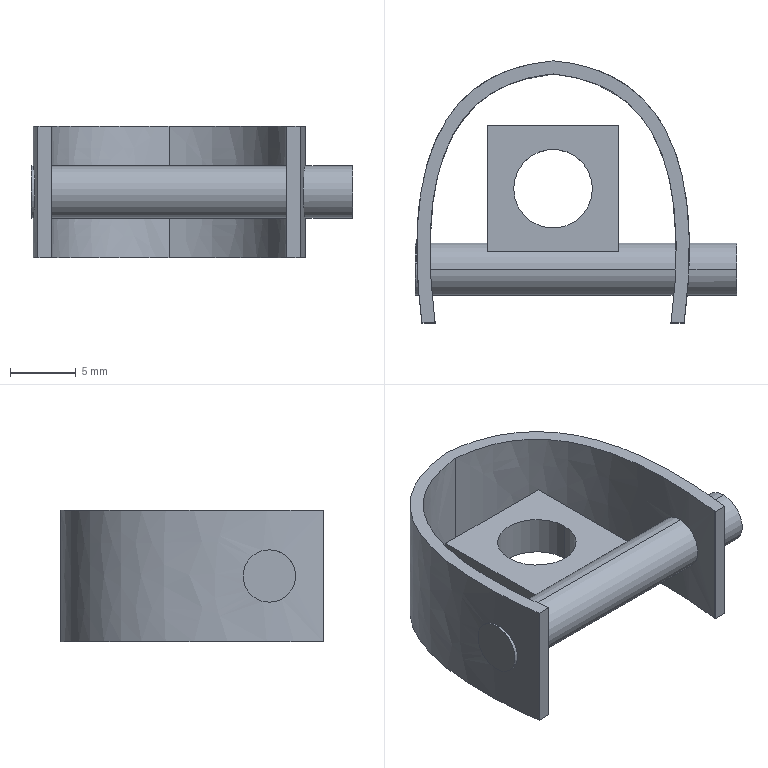Part | SolidWorks | features ICE 4, Extrusion 1 | 1 solid | 25 faces | box 24.5 x 20 x 10 mm | volume 968.354 mm3 | plane 11 | cylinder 10 | spline 4 | commonest cylinder face diameters 4 x6 6 x2 0.56 x1 0.938 x1
STEP:
#1=CARTESIAN_POINT('',(-3.,10.247,3.5));
#2=VERTEX_POINT('',#1);
#3=CARTESIAN_POINT('',(3.,10.247,3.5));
#4=VERTEX_POINT('',#3);
#5=CARTESIAN_POINT('',(0.,10.247,3.5));
#6=DIRECTION('',(0.,0.,1.));
#7=DIRECTION('',(1.,0.,0.));
#8=AXIS2_PLACEMENT_3D('',#5,#6,#7);
#9=CIRCLE('',#8,3.);
#10=EDGE_CURVE('',#2,#4,#9,.T.);
#11=ORIENTED_EDGE('',*,*,#10,.F.);
#12=CARTESIAN_POINT('',(-3.,10.247,6.5));
#13=VERTEX_POINT('',#12);
#14=CARTESIAN_POINT('',(-3.,10.247,-10.5));
#15=DIRECTION('',(0.,0.,1.));
#16=VECTOR('',#15,1000.);
#17=LINE('',#14,#16);
#18=EDGE_CURVE('',#2,#13,#17,.T.);
#19=ORIENTED_EDGE('',*,*,#18,.T.);
#20=CARTESIAN_POINT('',(3.,10.247,6.5));
#21=VERTEX_POINT('',#20);
#22=CARTESIAN_POINT('',(0.,10.247,6.5));
#23=DIRECTION('',(0.,0.,1.));
#24=DIRECTION('',(1.,0.,0.));
#25=AXIS2_PLACEMENT_3D('',#22,#23,#24);
#26=CIRCLE('',#25,3.);
#27=EDGE_CURVE('',#13,#21,#26,.T.);
#28=ORIENTED_EDGE('',*,*,#27,.T.);
#29=CARTESIAN_POINT('',(3.,10.247,-10.5));
#30=DIRECTION('',(0.,0.,1.));
#31=VECTOR('',#30,1000.);
#32=LINE('',#29,#31);
#33=EDGE_CURVE('',#4,#21,#32,.T.);
#34=ORIENTED_EDGE('',*,*,#33,.F.);
#35=EDGE_LOOP('',(#11,#19,#28,#34));
#36=FACE_OUTER_BOUND('',#35,.T.);
#37=CARTESIAN_POINT('',(0.,10.247,-10.5));
#38=DIRECTION('',(0.,0.,1.));
#39=DIRECTION('',(1.,0.,0.));
#40=AXIS2_PLACEMENT_3D('',#37,#38,#39);
#41=CYLINDRICAL_SURFACE('',#40,3.);
#42=ADVANCED_FACE('',(#36),#41,.F.);
#43=CARTESIAN_POINT('',(-10.5,4.102,7.));
#44=VERTEX_POINT('',#43);
#45=CARTESIAN_POINT('',(-10.5,4.102,3.));
#46=VERTEX_POINT('',#45);
#47=CARTESIAN_POINT('',(-10.5,4.102,5.));
#48=DIRECTION('',(-1.,0.,0.));
#49=DIRECTION('',(0.,0.,1.));
#50=AXIS2_PLACEMENT_3D('',#47,#48,#49);
#51=CIRCLE('',#50,2.);
#52=EDGE_CURVE('',#44,#46,#51,.T.);
#53=ORIENTED_EDGE('',*,*,#52,.F.);
#54=CARTESIAN_POINT('',(-10.36,4.102,7.));
#55=VERTEX_POINT('',#54);
#56=CARTESIAN_POINT('',(-10.5,4.102,7.));
#57=DIRECTION('',(1.,0.,0.));
#58=VECTOR('',#57,1000.);
#59=LINE('',#56,#58);
#60=EDGE_CURVE('',#44,#55,#59,.T.);
#61=ORIENTED_EDGE('',*,*,#60,.T.);
#62=CARTESIAN_POINT('',(-10.36,4.102,3.));
#63=VERTEX_POINT('',#62);
#64=CARTESIAN_POINT('',(-10.36,4.102,7.));
#65=CARTESIAN_POINT('',(-10.371,4.363,7.));
#66=CARTESIAN_POINT('',(-10.379,4.626,6.948));
#67=CARTESIAN_POINT('',(-10.39,5.107,6.749));
#68=CARTESIAN_POINT('',(-10.393,5.33,6.6));
#69=CARTESIAN_POINT('',(-10.395,5.607,6.323));
#70=CARTESIAN_POINT('',(-10.395,5.692,6.22));
#71=CARTESIAN_POINT('',(-10.394,5.837,6.003));
#72=CARTESIAN_POINT('',(-10.394,5.899,5.888));
#73=CARTESIAN_POINT('',(-10.393,5.999,5.646));
#74=CARTESIAN_POINT('',(-10.393,6.038,5.519));
#75=CARTESIAN_POINT('',(-10.392,6.089,5.263));
#76=CARTESIAN_POINT('',(-10.392,6.102,5.134));
#77=CARTESIAN_POINT('',(-10.392,6.102,4.87));
#78=CARTESIAN_POINT('',(-10.392,6.089,4.739));
#79=CARTESIAN_POINT('',(-10.393,6.039,4.484));
#80=CARTESIAN_POINT('',(-10.393,6.,4.357));
#81=CARTESIAN_POINT('',(-10.394,5.9,4.114));
#82=CARTESIAN_POINT('',(-10.394,5.839,3.999));
#83=CARTESIAN_POINT('',(-10.395,5.694,3.782));
#84=CARTESIAN_POINT('',(-10.395,5.609,3.679));
#85=CARTESIAN_POINT('',(-10.394,5.425,3.494));
#86=CARTESIAN_POINT('',(-10.393,5.324,3.411));
#87=CARTESIAN_POINT('',(-10.39,5.106,3.265));
#88=CARTESIAN_POINT('',(-10.388,4.989,3.203));
#89=CARTESIAN_POINT('',(-10.379,4.628,3.053));
#90=CARTESIAN_POINT('',(-10.371,4.366,3.));
#91=CARTESIAN_POINT('',(-10.36,4.102,3.));
#92=B_SPLINE_CURVE_WITH_KNOTS('',3,(#64,#65,#66,#67,#68,#69,#70,#71,#72,#73,#74,#75,#76,#77,#78,#79,#80,#81,#82,#83,#84,#85,#86,#87,#88,#89,#90,#91),.UNSPECIFIED.,.F.,.F.,(4,2,2,2,2,2,2,2,2,2,2,2,2,4),(0.006259,0.007041,0.007822,0.008213,0.008604,0.008994,0.009385,0.009776,0.01017,0.01056,0.01095,0.01134,0.01173,0.01251),.UNSPECIFIED.);
#93=EDGE_CURVE('',#55,#63,#92,.T.);
#94=ORIENTED_EDGE('',*,*,#93,.T.);
#95=CARTESIAN_POINT('',(-10.5,4.102,3.));
#96=DIRECTION('',(1.,0.,0.));
#97=VECTOR('',#96,1000.);
#98=LINE('',#95,#97);
#99=EDGE_CURVE('',#46,#63,#98,.T.);
#100=ORIENTED_EDGE('',*,*,#99,.F.);
#101=EDGE_LOOP('',(#53,#61,#94,#100));
#102=FACE_OUTER_BOUND('',#101,.T.);
#103=CARTESIAN_POINT('',(-10.5,4.102,5.));
#104=DIRECTION('',(1.,0.,0.));
#105=DIRECTION('',(0.,0.,-1.));
#106=AXIS2_PLACEMENT_3D('',#103,#104,#105);
#107=CYLINDRICAL_SURFACE('',#106,2.);
#108=ADVANCED_FACE('',(#102),#107,.T.);
#109=CARTESIAN_POINT('',(5.,5.425,6.5));
#110=VERTEX_POINT('',#109);
#111=CARTESIAN_POINT('',(5.,5.425,3.5));
#112=VERTEX_POINT('',#111);
#113=CARTESIAN_POINT('',(5.,4.102,5.));
#114=DIRECTION('',(-1.,0.,0.));
#115=DIRECTION('',(0.,-1.,0.));
#116=AXIS2_PLACEMENT_3D('',#113,#114,#115);
#117=CIRCLE('',#116,2.);
#118=EDGE_CURVE('',#110,#112,#117,.T.);
#119=ORIENTED_EDGE('',*,*,#118,.F.);
#120=CARTESIAN_POINT('',(-5.,5.425,6.5));
#121=VERTEX_POINT('',#120);
#122=CARTESIAN_POINT('',(14.,5.425,6.5));
#123=DIRECTION('',(-1.,0.,0.));
#124=VECTOR('',#123,1000.);
#125=LINE('',#122,#124);
#126=EDGE_CURVE('',#110,#121,#125,.T.);
#127=ORIENTED_EDGE('',*,*,#126,.T.);
#128=CARTESIAN_POINT('',(-5.,5.425,3.5));
#129=VERTEX_POINT('',#128);
#130=CARTESIAN_POINT('',(-5.,4.102,5.));
#131=DIRECTION('',(1.,0.,0.));
#132=DIRECTION('',(0.,1.,0.));
#133=AXIS2_PLACEMENT_3D('',#130,#131,#132);
#134=CIRCLE('',#133,2.);
#135=EDGE_CURVE('',#129,#121,#134,.T.);
#136=ORIENTED_EDGE('',*,*,#135,.F.);
#137=CARTESIAN_POINT('',(14.,5.425,3.5));
#138=DIRECTION('',(-1.,0.,0.));
#139=VECTOR('',#138,1000.);
#140=LINE('',#137,#139);
#141=EDGE_CURVE('',#112,#129,#140,.T.);
#142=ORIENTED_EDGE('',*,*,#141,.F.);
#143=EDGE_LOOP('',(#119,#127,#136,#142));
#144=FACE_BOUND('',#143,.T.);
#145=CARTESIAN_POINT('',(9.359,4.102,7.));
#146=VERTEX_POINT('',#145);
#147=CARTESIAN_POINT('',(9.359,4.102,3.));
#148=VERTEX_POINT('',#147);
#149=CARTESIAN_POINT('',(9.359,4.102,7.));
#150=CARTESIAN_POINT('',(9.365,4.234,7.));
#151=CARTESIAN_POINT('',(9.37,4.364,6.987));
#152=CARTESIAN_POINT('',(9.378,4.619,6.936));
#153=CARTESIAN_POINT('',(9.382,4.746,6.898));
#154=CARTESIAN_POINT('',(9.388,4.989,6.797));
#155=CARTESIAN_POINT('',(9.39,5.103,6.736));
#156=CARTESIAN_POINT('',(9.393,5.321,6.591));
#157=CARTESIAN_POINT('',(9.394,5.424,6.506));
#158=CARTESIAN_POINT('',(9.395,5.701,6.23));
#159=CARTESIAN_POINT('',(9.394,5.85,6.006));
#160=CARTESIAN_POINT('',(9.393,6.049,5.525));
#161=CARTESIAN_POINT('',(9.392,6.102,5.262));
#162=CARTESIAN_POINT('',(9.392,6.102,4.87));
#163=CARTESIAN_POINT('',(9.392,6.089,4.738));
#164=CARTESIAN_POINT('',(9.393,6.038,4.481));
#165=CARTESIAN_POINT('',(9.393,6.,4.356));
#166=CARTESIAN_POINT('',(9.394,5.9,4.114));
#167=CARTESIAN_POINT('',(9.394,5.837,3.997));
#168=CARTESIAN_POINT('',(9.395,5.692,3.78));
#169=CARTESIAN_POINT('',(9.395,5.61,3.679));
#170=CARTESIAN_POINT('',(9.394,5.423,3.493));
#171=CARTESIAN_POINT('',(9.393,5.322,3.41));
#172=CARTESIAN_POINT('',(9.39,5.105,3.265));
#173=CARTESIAN_POINT('',(9.388,4.988,3.202));
#174=CARTESIAN_POINT('',(9.382,4.746,3.102));
#175=CARTESIAN_POINT('',(9.378,4.621,3.064));
#176=CARTESIAN_POINT('',(9.37,4.365,3.013));
#177=CARTESIAN_POINT('',(9.365,4.232,3.));
#178=CARTESIAN_POINT('',(9.359,4.102,3.));
#179=B_SPLINE_CURVE_WITH_KNOTS('',3,(#149,#150,#151,#152,#153,#154,#155,#156,#157,#158,#159,#160,#161,#162,#163,#164,#165,#166,#167,#168,#169,#170,#171,#172,#173,#174,#175,#176,#177,#178),.UNSPECIFIED.,.F.,.F.,(4,2,2,2,2,2,2,2,2,2,2,2,2,2,4),(0.,0.0003909,0.0007817,0.001173,0.001563,0.002345,0.003127,0.003518,0.003909,0.0043,0.00469,0.005081,0.005472,0.005863,0.006254),.UNSPECIFIED.);
#180=EDGE_CURVE('',#146,#148,#179,.T.);
#181=ORIENTED_EDGE('',*,*,#180,.T.);
#182=CARTESIAN_POINT('',(-9.359,4.102,3.));
#183=VERTEX_POINT('',#182);
#184=CARTESIAN_POINT('',(14.,4.102,3.));
#185=DIRECTION('',(-1.,0.,0.));
#186=VECTOR('',#185,1000.);
#187=LINE('',#184,#186);
#188=EDGE_CURVE('',#148,#183,#187,.T.);
#189=ORIENTED_EDGE('',*,*,#188,.T.);
#190=CARTESIAN_POINT('',(-9.359,4.102,7.));
#191=VERTEX_POINT('',#190);
#192=CARTESIAN_POINT('',(-9.359,4.102,3.));
#193=CARTESIAN_POINT('',(-9.365,4.234,3.));
#194=CARTESIAN_POINT('',(-9.37,4.364,3.013));
#195=CARTESIAN_POINT('',(-9.378,4.619,3.064));
#196=CARTESIAN_POINT('',(-9.382,4.746,3.102));
#197=CARTESIAN_POINT('',(-9.388,4.989,3.203));
#198=CARTESIAN_POINT('',(-9.39,5.103,3.264));
#199=CARTESIAN_POINT('',(-9.393,5.321,3.409));
#200=CARTESIAN_POINT('',(-9.394,5.424,3.494));
#201=CARTESIAN_POINT('',(-9.395,5.701,3.77));
#202=CARTESIAN_POINT('',(-9.394,5.85,3.994));
#203=CARTESIAN_POINT('',(-9.393,6.049,4.475));
#204=CARTESIAN_POINT('',(-9.392,6.102,4.738));
#205=CARTESIAN_POINT('',(-9.392,6.102,5.13));
#206=CARTESIAN_POINT('',(-9.392,6.089,5.262));
#207=CARTESIAN_POINT('',(-9.393,6.038,5.519));
#208=CARTESIAN_POINT('',(-9.393,6.,5.644));
#209=CARTESIAN_POINT('',(-9.394,5.9,5.886));
#210=CARTESIAN_POINT('',(-9.394,5.837,6.003));
#211=CARTESIAN_POINT('',(-9.395,5.692,6.22));
#212=CARTESIAN_POINT('',(-9.395,5.61,6.321));
#213=CARTESIAN_POINT('',(-9.394,5.423,6.507));
#214=CARTESIAN_POINT('',(-9.393,5.322,6.59));
#215=CARTESIAN_POINT('',(-9.39,5.105,6.735));
#216=CARTESIAN_POINT('',(-9.388,4.988,6.798));
#217=CARTESIAN_POINT('',(-9.382,4.746,6.898));
#218=CARTESIAN_POINT('',(-9.378,4.621,6.936));
#219=CARTESIAN_POINT('',(-9.37,4.365,6.987));
#220=CARTESIAN_POINT('',(-9.365,4.232,7.));
#221=CARTESIAN_POINT('',(-9.359,4.102,7.));
#222=B_SPLINE_CURVE_WITH_KNOTS('',3,(#192,#193,#194,#195,#196,#197,#198,#199,#200,#201,#202,#203,#204,#205,#206,#207,#208,#209,#210,#211,#212,#213,#214,#215,#216,#217,#218,#219,#220,#221),.UNSPECIFIED.,.F.,.F.,(4,2,2,2,2,2,2,2,2,2,2,2,2,2,4),(0.,0.0003909,0.0007817,0.001173,0.001563,0.002345,0.003127,0.003518,0.003909,0.0043,0.00469,0.005081,0.005472,0.005863,0.006254),.UNSPECIFIED.);
#223=EDGE_CURVE('',#183,#191,#222,.T.);
#224=ORIENTED_EDGE('',*,*,#223,.T.);
#225=CARTESIAN_POINT('',(14.,4.102,7.));
#226=DIRECTION('',(-1.,0.,0.));
#227=VECTOR('',#226,1000.);
#228=LINE('',#225,#227);
#229=EDGE_CURVE('',#146,#191,#228,.T.);
#230=ORIENTED_EDGE('',*,*,#229,.F.);
#231=EDGE_LOOP('',(#181,#189,#224,#230));
#232=FACE_OUTER_BOUND('',#231,.T.);
#233=CARTESIAN_POINT('',(14.,4.102,5.));
#234=DIRECTION('',(-1.,0.,0.));
#235=DIRECTION('',(0.,0.,1.));
#236=AXIS2_PLACEMENT_3D('',#233,#234,#235);
#237=CYLINDRICAL_SURFACE('',#236,2.);
#238=ADVANCED_FACE('',(#144,#232),#237,.T.);
#239=CARTESIAN_POINT('',(14.,4.102,3.));
#240=VERTEX_POINT('',#239);
#241=CARTESIAN_POINT('',(14.,4.102,7.));
#242=VERTEX_POINT('',#241);
#243=CARTESIAN_POINT('',(14.,4.102,5.));
#244=DIRECTION('',(1.,0.,0.));
#245=DIRECTION('',(0.,0.,-1.));
#246=AXIS2_PLACEMENT_3D('',#243,#244,#245);
#247=CIRCLE('',#246,2.);
#248=EDGE_CURVE('',#240,#242,#247,.T.);
#249=ORIENTED_EDGE('',*,*,#248,.F.);
#250=CARTESIAN_POINT('',(10.36,4.102,3.));
#251=VERTEX_POINT('',#250);
#252=CARTESIAN_POINT('',(14.,4.102,3.));
#253=DIRECTION('',(-1.,0.,0.));
#254=VECTOR('',#253,1000.);
#255=LINE('',#252,#254);
#256=EDGE_CURVE('',#240,#251,#255,.T.);
#257=ORIENTED_EDGE('',*,*,#256,.T.);
#258=CARTESIAN_POINT('',(10.36,4.102,7.));
#259=VERTEX_POINT('',#258);
#260=CARTESIAN_POINT('',(10.36,4.102,3.));
#261=CARTESIAN_POINT('',(10.371,4.363,3.));
#262=CARTESIAN_POINT('',(10.379,4.626,3.052));
#263=CARTESIAN_POINT('',(10.39,5.107,3.251));
#264=CARTESIAN_POINT('',(10.393,5.33,3.4));
#265=CARTESIAN_POINT('',(10.395,5.607,3.677));
#266=CARTESIAN_POINT('',(10.395,5.692,3.78));
#267=CARTESIAN_POINT('',(10.394,5.837,3.997));
#268=CARTESIAN_POINT('',(10.394,5.899,4.112));
#269=CARTESIAN_POINT('',(10.393,5.999,4.354));
#270=CARTESIAN_POINT('',(10.393,6.038,4.481));
#271=CARTESIAN_POINT('',(10.392,6.089,4.737));
#272=CARTESIAN_POINT('',(10.392,6.102,4.866));
#273=CARTESIAN_POINT('',(10.392,6.102,5.13));
#274=CARTESIAN_POINT('',(10.392,6.089,5.261));
#275=CARTESIAN_POINT('',(10.393,6.039,5.516));
#276=CARTESIAN_POINT('',(10.393,6.,5.643));
#277=CARTESIAN_POINT('',(10.394,5.9,5.886));
#278=CARTESIAN_POINT('',(10.394,5.839,6.001));
#279=CARTESIAN_POINT('',(10.395,5.694,6.218));
#280=CARTESIAN_POINT('',(10.395,5.609,6.321));
#281=CARTESIAN_POINT('',(10.394,5.425,6.506));
#282=CARTESIAN_POINT('',(10.393,5.324,6.589));
#283=CARTESIAN_POINT('',(10.39,5.106,6.735));
#284=CARTESIAN_POINT('',(10.388,4.989,6.797));
#285=CARTESIAN_POINT('',(10.379,4.628,6.947));
#286=CARTESIAN_POINT('',(10.371,4.366,7.));
#287=CARTESIAN_POINT('',(10.36,4.102,7.));
#288=B_SPLINE_CURVE_WITH_KNOTS('',3,(#260,#261,#262,#263,#264,#265,#266,#267,#268,#269,#270,#271,#272,#273,#274,#275,#276,#277,#278,#279,#280,#281,#282,#283,#284,#285,#286,#287),.UNSPECIFIED.,.F.,.F.,(4,2,2,2,2,2,2,2,2,2,2,2,2,4),(0.006259,0.007041,0.007822,0.008213,0.008604,0.008994,0.009385,0.009776,0.01017,0.01056,0.01095,0.01134,0.01173,0.01251),.UNSPECIFIED.);
#289=EDGE_CURVE('',#251,#259,#288,.T.);
#290=ORIENTED_EDGE('',*,*,#289,.T.);
#291=CARTESIAN_POINT('',(14.,4.102,7.));
#292=DIRECTION('',(-1.,0.,0.));
#293=VECTOR('',#292,1000.);
#294=LINE('',#291,#293);
#295=EDGE_CURVE('',#242,#259,#294,.T.);
#296=ORIENTED_EDGE('',*,*,#295,.F.);
#297=EDGE_LOOP('',(#249,#257,#290,#296));
#298=FACE_OUTER_BOUND('',#297,.T.);
#299=CARTESIAN_POINT('',(14.,4.102,5.));
#300=DIRECTION('',(-1.,0.,0.));
#301=DIRECTION('',(0.,0.,1.));
#302=AXIS2_PLACEMENT_3D('',#299,#300,#301);
#303=CYLINDRICAL_SURFACE('',#302,2.);
#304=ADVANCED_FACE('',(#298),#303,.T.);
#305=CARTESIAN_POINT('',(0.,20.,0.));
#306=VERTEX_POINT('',#305);
#307=CARTESIAN_POINT('',(-10.,0.,0.));
#308=VERTEX_POINT('',#307);
#309=CARTESIAN_POINT('',(0.,20.,0.));
#310=CARTESIAN_POINT('',(-12.419,18.909,0.));
#311=CARTESIAN_POINT('',(-10.,0.,0.));
#312=B_SPLINE_CURVE_WITH_KNOTS('',2,(#309,#310,#311),.UNSPECIFIED.,.F.,.F.,(3,3),(0.,1.),.UNSPECIFIED.);
#313=EDGE_CURVE('',#306,#308,#312,.T.);
#314=ORIENTED_EDGE('',*,*,#313,.T.);
#315=CARTESIAN_POINT('',(-10.,0.,10.));
#316=VERTEX_POINT('',#315);
#317=CARTESIAN_POINT('',(-10.,0.,10.));
#318=DIRECTION('',(0.,0.,-1.));
#319=VECTOR('',#318,1000.);
#320=LINE('',#317,#319);
#321=EDGE_CURVE('',#316,#308,#320,.T.);
#322=ORIENTED_EDGE('',*,*,#321,.F.);
#323=CARTESIAN_POINT('',(0.,20.,10.));
#324=VERTEX_POINT('',#323);
#325=CARTESIAN_POINT('',(0.,20.,10.));
#326=CARTESIAN_POINT('',(-12.419,18.909,10.));
#327=CARTESIAN_POINT('',(-10.,0.,10.));
#328=B_SPLINE_CURVE_WITH_KNOTS('',2,(#325,#326,#327),.UNSPECIFIED.,.F.,.F.,(3,3),(0.,1.),.UNSPECIFIED.);
#329=EDGE_CURVE('',#324,#316,#328,.T.);
#330=ORIENTED_EDGE('',*,*,#329,.F.);
#331=CARTESIAN_POINT('',(0.,20.,10.));
#332=DIRECTION('',(0.,0.,-1.));
#333=VECTOR('',#332,1000.);
#334=LINE('',#331,#333);
#335=EDGE_CURVE('',#324,#306,#334,.T.);
#336=ORIENTED_EDGE('',*,*,#335,.T.);
#337=EDGE_LOOP('',(#314,#322,#330,#336));
#338=FACE_OUTER_BOUND('',#337,.T.);
#339=CARTESIAN_POINT('',(-10.36,4.102,3.));
#340=CARTESIAN_POINT('',(-10.354,3.97,3.));
#341=CARTESIAN_POINT('',(-10.348,3.84,3.013));
#342=CARTESIAN_POINT('',(-10.335,3.584,3.064));
#343=CARTESIAN_POINT('',(-10.327,3.457,3.102));
#344=CARTESIAN_POINT('',(-10.313,3.215,3.203));
#345=CARTESIAN_POINT('',(-10.305,3.1,3.264));
#346=CARTESIAN_POINT('',(-10.29,2.883,3.409));
#347=CARTESIAN_POINT('',(-10.283,2.78,3.493));
#348=CARTESIAN_POINT('',(-10.262,2.503,3.77));
#349=CARTESIAN_POINT('',(-10.25,2.354,3.993));
#350=CARTESIAN_POINT('',(-10.233,2.155,4.475));
#351=CARTESIAN_POINT('',(-10.228,2.102,4.738));
#352=CARTESIAN_POINT('',(-10.228,2.102,5.13));
#353=CARTESIAN_POINT('',(-10.229,2.115,5.262));
#354=CARTESIAN_POINT('',(-10.234,2.166,5.519));
#355=CARTESIAN_POINT('',(-10.237,2.204,5.644));
#356=CARTESIAN_POINT('',(-10.245,2.304,5.886));
#357=CARTESIAN_POINT('',(-10.251,2.367,6.003));
#358=CARTESIAN_POINT('',(-10.262,2.512,6.22));
#359=CARTESIAN_POINT('',(-10.269,2.594,6.321));
#360=CARTESIAN_POINT('',(-10.283,2.781,6.508));
#361=CARTESIAN_POINT('',(-10.29,2.882,6.59));
#362=CARTESIAN_POINT('',(-10.305,3.099,6.735));
#363=CARTESIAN_POINT('',(-10.313,3.216,6.798));
#364=CARTESIAN_POINT('',(-10.327,3.458,6.898));
#365=CARTESIAN_POINT('',(-10.335,3.583,6.936));
#366=CARTESIAN_POINT('',(-10.348,3.839,6.987));
#367=CARTESIAN_POINT('',(-10.354,3.971,7.));
#368=CARTESIAN_POINT('',(-10.36,4.102,7.));
#369=B_SPLINE_CURVE_WITH_KNOTS('',3,(#339,#340,#341,#342,#343,#344,#345,#346,#347,#348,#349,#350,#351,#352,#353,#354,#355,#356,#357,#358,#359,#360,#361,#362,#363,#364,#365,#366,#367,#368),.UNSPECIFIED.,.F.,.F.,(4,2,2,2,2,2,2,2,2,2,2,2,2,2,4),(0.,0.0003912,0.0007824,0.001174,0.001565,0.002347,0.00313,0.003521,0.003912,0.004303,0.004694,0.005086,0.005477,0.005868,0.006259),.UNSPECIFIED.);
#370=EDGE_CURVE('',#63,#55,#369,.T.);
#371=ORIENTED_EDGE('',*,*,#370,.F.);
#372=ORIENTED_EDGE('',*,*,#93,.F.);
#373=EDGE_LOOP('',(#371,#372));
#374=FACE_BOUND('',#373,.T.);
#375=CARTESIAN_POINT('',(0.,20.,10.));
#376=CARTESIAN_POINT('',(0.,20.,0.));
#377=CARTESIAN_POINT('',(-12.419,18.909,10.));
#378=CARTESIAN_POINT('',(-12.419,18.909,0.));
#379=CARTESIAN_POINT('',(-10.,0.,10.));
#380=CARTESIAN_POINT('',(-10.,0.,0.));
#381=B_SPLINE_SURFACE_WITH_KNOTS('',2,1,((#375,#376),(#377,#378),(#379,#380)),.UNSPECIFIED.,.F.,.F.,.F.,(3,3),(2,2),(0.,1.),(0.,1.),.UNSPECIFIED.);
#382=ADVANCED_FACE('',(#338,#374),#381,.F.);
#383=CARTESIAN_POINT('',(-9.008,0.1269,0.));
#384=VERTEX_POINT('',#383);
#385=CARTESIAN_POINT('',(0.,18.996,0.));
#386=VERTEX_POINT('',#385);
#387=CARTESIAN_POINT('',(-9.008,0.1269,0.));
#388=CARTESIAN_POINT('',(-9.057,0.5062,0.));
#389=CARTESIAN_POINT('',(-9.147,1.275,0.));
#390=CARTESIAN_POINT('',(-9.287,2.741,0.));
#391=CARTESIAN_POINT('',(-9.392,4.492,0.));
#392=CARTESIAN_POINT('',(-9.405,6.444,0.));
#393=CARTESIAN_POINT('',(-9.274,8.852,0.));
#394=CARTESIAN_POINT('',(-8.837,11.493,0.));
#395=CARTESIAN_POINT('',(-7.897,14.069,0.));
#396=CARTESIAN_POINT('',(-6.57,16.069,0.));
#397=CARTESIAN_POINT('',(-4.863,17.548,0.));
#398=CARTESIAN_POINT('',(-3.071,18.387,0.));
#399=CARTESIAN_POINT('',(-1.41,18.817,0.));
#400=CARTESIAN_POINT('',(-0.463,18.953,0.));
#401=CARTESIAN_POINT('',(0.,18.996,0.));
#402=B_SPLINE_CURVE_WITH_KNOTS('',3,(#387,#388,#389,#390,#391,#392,#393,#394,#395,#396,#397,#398,#399,#400,#401),.UNSPECIFIED.,.F.,.F.,(4,1,1,1,1,1,1,1,1,1,1,1,4),(0.003764,0.0349,0.06603,0.1283,0.1906,0.2528,0.3774,0.5019,0.6264,0.7509,0.8755,0.9377,1.),.UNSPECIFIED.);
#403=EDGE_CURVE('',#384,#386,#402,.T.);
#404=ORIENTED_EDGE('',*,*,#403,.T.);
#405=CARTESIAN_POINT('',(0.,18.996,10.));
#406=VERTEX_POINT('',#405);
#407=CARTESIAN_POINT('',(0.,18.996,10.));
#408=DIRECTION('',(0.,0.,-1.));
#409=VECTOR('',#408,1000.);
#410=LINE('',#407,#409);
#411=EDGE_CURVE('',#406,#386,#410,.T.);
#412=ORIENTED_EDGE('',*,*,#411,.F.);
#413=CARTESIAN_POINT('',(-9.008,0.1269,10.));
#414=VERTEX_POINT('',#413);
#415=CARTESIAN_POINT('',(-9.008,0.1269,10.));
#416=CARTESIAN_POINT('',(-9.057,0.5062,10.));
#417=CARTESIAN_POINT('',(-9.147,1.275,10.));
#418=CARTESIAN_POINT('',(-9.287,2.741,10.));
#419=CARTESIAN_POINT('',(-9.392,4.492,10.));
#420=CARTESIAN_POINT('',(-9.405,6.444,10.));
#421=CARTESIAN_POINT('',(-9.274,8.852,10.));
#422=CARTESIAN_POINT('',(-8.837,11.493,10.));
#423=CARTESIAN_POINT('',(-7.897,14.069,10.));
#424=CARTESIAN_POINT('',(-6.57,16.069,10.));
#425=CARTESIAN_POINT('',(-4.863,17.548,10.));
#426=CARTESIAN_POINT('',(-3.071,18.387,10.));
#427=CARTESIAN_POINT('',(-1.41,18.817,10.));
#428=CARTESIAN_POINT('',(-0.463,18.953,10.));
#429=CARTESIAN_POINT('',(0.,18.996,10.));
#430=B_SPLINE_CURVE_WITH_KNOTS('',3,(#415,#416,#417,#418,#419,#420,#421,#422,#423,#424,#425,#426,#427,#428,#429),.UNSPECIFIED.,.F.,.F.,(4,1,1,1,1,1,1,1,1,1,1,1,4),(0.003764,0.0349,0.06603,0.1283,0.1906,0.2528,0.3774,0.5019,0.6264,0.7509,0.8755,0.9377,1.),.UNSPECIFIED.);
#431=EDGE_CURVE('',#414,#406,#430,.T.);
#432=ORIENTED_EDGE('',*,*,#431,.F.);
#433=CARTESIAN_POINT('',(-9.008,0.1269,10.));
#434=DIRECTION('',(0.,0.,-1.));
#435=VECTOR('',#434,1000.);
#436=LINE('',#433,#435);
#437=EDGE_CURVE('',#414,#384,#436,.T.);
#438=ORIENTED_EDGE('',*,*,#437,.T.);
#439=EDGE_LOOP('',(#404,#412,#432,#438));
#440=FACE_OUTER_BOUND('',#439,.T.);
#441=CARTESIAN_POINT('',(-9.359,4.102,7.));
#442=CARTESIAN_POINT('',(-9.347,3.841,7.));
#443=CARTESIAN_POINT('',(-9.333,3.578,6.948));
#444=CARTESIAN_POINT('',(-9.303,3.097,6.749));
#445=CARTESIAN_POINT('',(-9.287,2.874,6.6));
#446=CARTESIAN_POINT('',(-9.266,2.597,6.324));
#447=CARTESIAN_POINT('',(-9.259,2.512,6.221));
#448=CARTESIAN_POINT('',(-9.247,2.367,6.004));
#449=CARTESIAN_POINT('',(-9.242,2.305,5.889));
#450=CARTESIAN_POINT('',(-9.233,2.205,5.647));
#451=CARTESIAN_POINT('',(-9.23,2.166,5.52));
#452=CARTESIAN_POINT('',(-9.225,2.115,5.264));
#453=CARTESIAN_POINT('',(-9.224,2.102,5.134));
#454=CARTESIAN_POINT('',(-9.224,2.102,4.87));
#455=CARTESIAN_POINT('',(-9.225,2.115,4.739));
#456=CARTESIAN_POINT('',(-9.23,2.165,4.483));
#457=CARTESIAN_POINT('',(-9.233,2.204,4.356));
#458=CARTESIAN_POINT('',(-9.242,2.304,4.114));
#459=CARTESIAN_POINT('',(-9.247,2.366,3.999));
#460=CARTESIAN_POINT('',(-9.259,2.511,3.782));
#461=CARTESIAN_POINT('',(-9.266,2.595,3.679));
#462=CARTESIAN_POINT('',(-9.28,2.779,3.494));
#463=CARTESIAN_POINT('',(-9.287,2.88,3.411));
#464=CARTESIAN_POINT('',(-9.303,3.098,3.265));
#465=CARTESIAN_POINT('',(-9.311,3.215,3.203));
#466=CARTESIAN_POINT('',(-9.333,3.575,3.053));
#467=CARTESIAN_POINT('',(-9.347,3.838,3.));
#468=CARTESIAN_POINT('',(-9.359,4.102,3.));
#469=B_SPLINE_CURVE_WITH_KNOTS('',3,(#441,#442,#443,#444,#445,#446,#447,#448,#449,#450,#451,#452,#453,#454,#455,#456,#457,#458,#459,#460,#461,#462,#463,#464,#465,#466,#467,#468),.UNSPECIFIED.,.F.,.F.,(4,2,2,2,2,2,2,2,2,2,2,2,2,4),(0.006254,0.007036,0.007819,0.00821,0.008601,0.008992,0.009383,0.009774,0.01017,0.01056,0.01095,0.01134,0.01173,0.01251),.UNSPECIFIED.);
#470=EDGE_CURVE('',#191,#183,#469,.T.);
#471=ORIENTED_EDGE('',*,*,#470,.F.);
#472=ORIENTED_EDGE('',*,*,#223,.F.);
#473=EDGE_LOOP('',(#471,#472));
#474=FACE_BOUND('',#473,.T.);
#475=CARTESIAN_POINT('',(-9.008,0.1269,10.));
#476=CARTESIAN_POINT('',(-9.008,0.1269,0.));
#477=CARTESIAN_POINT('',(-9.057,0.5062,10.));
#478=CARTESIAN_POINT('',(-9.057,0.5062,0.));
#479=CARTESIAN_POINT('',(-9.147,1.275,10.));
#480=CARTESIAN_POINT('',(-9.147,1.275,0.));
#481=CARTESIAN_POINT('',(-9.287,2.741,10.));
#482=CARTESIAN_POINT('',(-9.287,2.741,0.));
#483=CARTESIAN_POINT('',(-9.392,4.492,10.));
#484=CARTESIAN_POINT('',(-9.392,4.492,0.));
#485=CARTESIAN_POINT('',(-9.405,6.444,10.));
#486=CARTESIAN_POINT('',(-9.405,6.444,0.));
#487=CARTESIAN_POINT('',(-9.274,8.852,10.));
#488=CARTESIAN_POINT('',(-9.274,8.852,0.));
#489=CARTESIAN_POINT('',(-8.837,11.493,10.));
#490=CARTESIAN_POINT('',(-8.837,11.493,0.));
#491=CARTESIAN_POINT('',(-7.897,14.069,10.));
#492=CARTESIAN_POINT('',(-7.897,14.069,0.));
#493=CARTESIAN_POINT('',(-6.57,16.069,10.));
#494=CARTESIAN_POINT('',(-6.57,16.069,0.));
#495=CARTESIAN_POINT('',(-4.863,17.548,10.));
#496=CARTESIAN_POINT('',(-4.863,17.548,0.));
#497=CARTESIAN_POINT('',(-3.071,18.387,10.));
#498=CARTESIAN_POINT('',(-3.071,18.387,0.));
#499=CARTESIAN_POINT('',(-1.41,18.817,10.));
#500=CARTESIAN_POINT('',(-1.41,18.817,0.));
#501=CARTESIAN_POINT('',(-0.463,18.953,10.));
#502=CARTESIAN_POINT('',(-0.463,18.953,0.));
#503=CARTESIAN_POINT('',(0.,18.996,10.));
#504=CARTESIAN_POINT('',(0.,18.996,0.));
#505=B_SPLINE_SURFACE_WITH_KNOTS('',3,1,((#475,#476),(#477,#478),(#479,#480),(#481,#482),(#483,#484),(#485,#486),(#487,#488),(#489,#490),(#491,#492),(#493,#494),(#495,#496),(#497,#498),(#499,#500),(#501,#502),(#503,#504)),.UNSPECIFIED.,.F.,.F.,.F.,(4,1,1,1,1,1,1,1,1,1,1,1,4),(2,2),(0.003764,0.0349,0.06603,0.1283,0.1906,0.2528,0.3774,0.5019,0.6264,0.7509,0.8755,0.9377,1.),(0.,1.),.UNSPECIFIED.);
#506=ADVANCED_FACE('',(#440,#474),#505,.F.);
#507=CARTESIAN_POINT('',(9.008,0.1269,0.));
#508=VERTEX_POINT('',#507);
#509=CARTESIAN_POINT('',(0.,18.996,0.));
#510=CARTESIAN_POINT('',(0.463,18.953,0.));
#511=CARTESIAN_POINT('',(1.41,18.817,0.));
#512=CARTESIAN_POINT('',(3.071,18.387,0.));
#513=CARTESIAN_POINT('',(4.863,17.548,0.));
#514=CARTESIAN_POINT('',(6.57,16.069,0.));
#515=CARTESIAN_POINT('',(7.897,14.069,0.));
#516=CARTESIAN_POINT('',(8.837,11.493,0.));
#517=CARTESIAN_POINT('',(9.274,8.852,0.));
#518=CARTESIAN_POINT('',(9.405,6.444,0.));
#519=CARTESIAN_POINT('',(9.392,4.492,0.));
#520=CARTESIAN_POINT('',(9.287,2.741,0.));
#521=CARTESIAN_POINT('',(9.147,1.275,0.));
#522=CARTESIAN_POINT('',(9.057,0.5062,0.));
#523=CARTESIAN_POINT('',(9.008,0.1269,0.));
#524=B_SPLINE_CURVE_WITH_KNOTS('',3,(#509,#510,#511,#512,#513,#514,#515,#516,#517,#518,#519,#520,#521,#522,#523),.UNSPECIFIED.,.F.,.F.,(4,1,1,1,1,1,1,1,1,1,1,1,4),(0.003764,0.06603,0.1283,0.2528,0.3774,0.5019,0.6264,0.7509,0.8132,0.8755,0.9377,0.9689,1.),.UNSPECIFIED.);
#525=EDGE_CURVE('',#386,#508,#524,.T.);
#526=ORIENTED_EDGE('',*,*,#525,.T.);
#527=CARTESIAN_POINT('',(9.008,0.1269,10.));
#528=VERTEX_POINT('',#527);
#529=CARTESIAN_POINT('',(9.008,0.1269,10.));
#530=DIRECTION('',(0.,0.,-1.));
#531=VECTOR('',#530,1000.);
#532=LINE('',#529,#531);
#533=EDGE_CURVE('',#528,#508,#532,.T.);
#534=ORIENTED_EDGE('',*,*,#533,.F.);
#535=CARTESIAN_POINT('',(0.,18.996,10.));
#536=CARTESIAN_POINT('',(0.463,18.953,10.));
#537=CARTESIAN_POINT('',(1.41,18.817,10.));
#538=CARTESIAN_POINT('',(3.071,18.387,10.));
#539=CARTESIAN_POINT('',(4.863,17.548,10.));
#540=CARTESIAN_POINT('',(6.57,16.069,10.));
#541=CARTESIAN_POINT('',(7.897,14.069,10.));
#542=CARTESIAN_POINT('',(8.837,11.493,10.));
#543=CARTESIAN_POINT('',(9.274,8.852,10.));
#544=CARTESIAN_POINT('',(9.405,6.444,10.));
#545=CARTESIAN_POINT('',(9.392,4.492,10.));
#546=CARTESIAN_POINT('',(9.287,2.741,10.));
#547=CARTESIAN_POINT('',(9.147,1.275,10.));
#548=CARTESIAN_POINT('',(9.057,0.5062,10.));
#549=CARTESIAN_POINT('',(9.008,0.1269,10.));
#550=B_SPLINE_CURVE_WITH_KNOTS('',3,(#535,#536,#537,#538,#539,#540,#541,#542,#543,#544,#545,#546,#547,#548,#549),.UNSPECIFIED.,.F.,.F.,(4,1,1,1,1,1,1,1,1,1,1,1,4),(0.003764,0.06603,0.1283,0.2528,0.3774,0.5019,0.6264,0.7509,0.8132,0.8755,0.9377,0.9689,1.),.UNSPECIFIED.);
#551=EDGE_CURVE('',#406,#528,#550,.T.);
#552=ORIENTED_EDGE('',*,*,#551,.F.);
#553=ORIENTED_EDGE('',*,*,#411,.T.);
#554=EDGE_LOOP('',(#526,#534,#552,#553));
#555=FACE_OUTER_BOUND('',#554,.T.);
#556=ORIENTED_EDGE('',*,*,#180,.F.);
#557=CARTESIAN_POINT('',(9.359,4.102,3.));
#558=CARTESIAN_POINT('',(9.347,3.841,3.));
#559=CARTESIAN_POINT('',(9.333,3.578,3.052));
#560=CARTESIAN_POINT('',(9.303,3.097,3.251));
#561=CARTESIAN_POINT('',(9.287,2.874,3.4));
#562=CARTESIAN_POINT('',(9.266,2.597,3.676));
#563=CARTESIAN_POINT('',(9.259,2.512,3.779));
#564=CARTESIAN_POINT('',(9.247,2.367,3.996));
#565=CARTESIAN_POINT('',(9.242,2.305,4.111));
#566=CARTESIAN_POINT('',(9.233,2.205,4.353));
#567=CARTESIAN_POINT('',(9.23,2.166,4.48));
#568=CARTESIAN_POINT('',(9.225,2.115,4.736));
#569=CARTESIAN_POINT('',(9.224,2.102,4.866));
#570=CARTESIAN_POINT('',(9.224,2.102,5.13));
#571=CARTESIAN_POINT('',(9.225,2.115,5.261));
#572=CARTESIAN_POINT('',(9.23,2.165,5.517));
#573=CARTESIAN_POINT('',(9.233,2.204,5.644));
#574=CARTESIAN_POINT('',(9.242,2.304,5.886));
#575=CARTESIAN_POINT('',(9.247,2.366,6.001));
#576=CARTESIAN_POINT('',(9.259,2.511,6.218));
#577=CARTESIAN_POINT('',(9.266,2.595,6.321));
#578=CARTESIAN_POINT('',(9.28,2.779,6.506));
#579=CARTESIAN_POINT('',(9.287,2.88,6.589));
#580=CARTESIAN_POINT('',(9.303,3.098,6.735));
#581=CARTESIAN_POINT('',(9.311,3.215,6.797));
#582=CARTESIAN_POINT('',(9.333,3.575,6.947));
#583=CARTESIAN_POINT('',(9.347,3.838,7.));
#584=CARTESIAN_POINT('',(9.359,4.102,7.));
#585=B_SPLINE_CURVE_WITH_KNOTS('',3,(#557,#558,#559,#560,#561,#562,#563,#564,#565,#566,#567,#568,#569,#570,#571,#572,#573,#574,#575,#576,#577,#578,#579,#580,#581,#582,#583,#584),.UNSPECIFIED.,.F.,.F.,(4,2,2,2,2,2,2,2,2,2,2,2,2,4),(0.006254,0.007036,0.007819,0.00821,0.008601,0.008992,0.009383,0.009774,0.01017,0.01056,0.01095,0.01134,0.01173,0.01251),.UNSPECIFIED.);
#586=EDGE_CURVE('',#148,#146,#585,.T.);
#587=ORIENTED_EDGE('',*,*,#586,.F.);
#588=EDGE_LOOP('',(#556,#587));
#589=FACE_BOUND('',#588,.T.);
#590=CARTESIAN_POINT('',(0.,18.996,10.));
#591=CARTESIAN_POINT('',(0.,18.996,0.));
#592=CARTESIAN_POINT('',(0.463,18.953,10.));
#593=CARTESIAN_POINT('',(0.463,18.953,0.));
#594=CARTESIAN_POINT('',(1.41,18.817,10.));
#595=CARTESIAN_POINT('',(1.41,18.817,0.));
#596=CARTESIAN_POINT('',(3.071,18.387,10.));
#597=CARTESIAN_POINT('',(3.071,18.387,0.));
#598=CARTESIAN_POINT('',(4.863,17.548,10.));
#599=CARTESIAN_POINT('',(4.863,17.548,0.));
#600=CARTESIAN_POINT('',(6.57,16.069,10.));
#601=CARTESIAN_POINT('',(6.57,16.069,0.));
#602=CARTESIAN_POINT('',(7.897,14.069,10.));
#603=CARTESIAN_POINT('',(7.897,14.069,0.));
#604=CARTESIAN_POINT('',(8.837,11.493,10.));
#605=CARTESIAN_POINT('',(8.837,11.493,0.));
#606=CARTESIAN_POINT('',(9.274,8.852,10.));
#607=CARTESIAN_POINT('',(9.274,8.852,0.));
#608=CARTESIAN_POINT('',(9.405,6.444,10.));
#609=CARTESIAN_POINT('',(9.405,6.444,0.));
#610=CARTESIAN_POINT('',(9.392,4.492,10.));
#611=CARTESIAN_POINT('',(9.392,4.492,0.));
#612=CARTESIAN_POINT('',(9.287,2.741,10.));
#613=CARTESIAN_POINT('',(9.287,2.741,0.));
#614=CARTESIAN_POINT('',(9.147,1.275,10.));
#615=CARTESIAN_POINT('',(9.147,1.275,0.));
#616=CARTESIAN_POINT('',(9.057,0.5062,10.));
#617=CARTESIAN_POINT('',(9.057,0.5062,0.));
#618=CARTESIAN_POINT('',(9.008,0.1269,10.));
#619=CARTESIAN_POINT('',(9.008,0.1269,0.));
#620=B_SPLINE_SURFACE_WITH_KNOTS('',3,1,((#590,#591),(#592,#593),(#594,#595),(#596,#597),(#598,#599),(#600,#601),(#602,#603),(#604,#605),(#606,#607),(#608,#609),(#610,#611),(#612,#613),(#614,#615),(#616,#617),(#618,#619)),.UNSPECIFIED.,.F.,.F.,.F.,(4,1,1,1,1,1,1,1,1,1,1,1,4),(2,2),(0.003764,0.06603,0.1283,0.2528,0.3774,0.5019,0.6264,0.7509,0.8132,0.8755,0.9377,0.9689,1.),(0.,1.),.UNSPECIFIED.);
#621=ADVANCED_FACE('',(#555,#589),#620,.F.);
#622=CARTESIAN_POINT('',(10.,0.,0.));
#623=VERTEX_POINT('',#622);
#624=CARTESIAN_POINT('',(10.,0.,0.));
#625=CARTESIAN_POINT('',(12.419,18.909,0.));
#626=CARTESIAN_POINT('',(0.,20.,0.));
#627=B_SPLINE_CURVE_WITH_KNOTS('',2,(#624,#625,#626),.UNSPECIFIED.,.F.,.F.,(3,3),(0.,1.),.UNSPECIFIED.);
#628=EDGE_CURVE('',#623,#306,#627,.T.);
#629=ORIENTED_EDGE('',*,*,#628,.T.);
#630=ORIENTED_EDGE('',*,*,#335,.F.);
#631=CARTESIAN_POINT('',(10.,0.,10.));
#632=VERTEX_POINT('',#631);
#633=CARTESIAN_POINT('',(10.,0.,10.));
#634=CARTESIAN_POINT('',(12.419,18.909,10.));
#635=CARTESIAN_POINT('',(0.,20.,10.));
#636=B_SPLINE_CURVE_WITH_KNOTS('',2,(#633,#634,#635),.UNSPECIFIED.,.F.,.F.,(3,3),(0.,1.),.UNSPECIFIED.);
#637=EDGE_CURVE('',#632,#324,#636,.T.);
#638=ORIENTED_EDGE('',*,*,#637,.F.);
#639=CARTESIAN_POINT('',(10.,0.,10.));
#640=DIRECTION('',(0.,0.,-1.));
#641=VECTOR('',#640,1000.);
#642=LINE('',#639,#641);
#643=EDGE_CURVE('',#632,#623,#642,.T.);
#644=ORIENTED_EDGE('',*,*,#643,.T.);
#645=EDGE_LOOP('',(#629,#630,#638,#644));
#646=FACE_OUTER_BOUND('',#645,.T.);
#647=CARTESIAN_POINT('',(10.36,4.102,7.));
#648=CARTESIAN_POINT('',(10.354,3.97,7.));
#649=CARTESIAN_POINT('',(10.348,3.84,6.987));
#650=CARTESIAN_POINT('',(10.335,3.584,6.936));
#651=CARTESIAN_POINT('',(10.327,3.457,6.898));
#652=CARTESIAN_POINT('',(10.313,3.215,6.797));
#653=CARTESIAN_POINT('',(10.305,3.1,6.736));
#654=CARTESIAN_POINT('',(10.29,2.883,6.591));
#655=CARTESIAN_POINT('',(10.283,2.78,6.507));
#656=CARTESIAN_POINT('',(10.262,2.503,6.23));
#657=CARTESIAN_POINT('',(10.25,2.354,6.007));
#658=CARTESIAN_POINT('',(10.233,2.155,5.525));
#659=CARTESIAN_POINT('',(10.228,2.102,5.262));
#660=CARTESIAN_POINT('',(10.228,2.102,4.87));
#661=CARTESIAN_POINT('',(10.229,2.115,4.738));
#662=CARTESIAN_POINT('',(10.234,2.166,4.481));
#663=CARTESIAN_POINT('',(10.237,2.204,4.356));
#664=CARTESIAN_POINT('',(10.245,2.304,4.114));
#665=CARTESIAN_POINT('',(10.251,2.367,3.997));
#666=CARTESIAN_POINT('',(10.262,2.512,3.78));
#667=CARTESIAN_POINT('',(10.269,2.594,3.679));
#668=CARTESIAN_POINT('',(10.283,2.781,3.492));
#669=CARTESIAN_POINT('',(10.29,2.882,3.41));
#670=CARTESIAN_POINT('',(10.305,3.099,3.265));
#671=CARTESIAN_POINT('',(10.313,3.216,3.202));
#672=CARTESIAN_POINT('',(10.327,3.458,3.102));
#673=CARTESIAN_POINT('',(10.335,3.583,3.064));
#674=CARTESIAN_POINT('',(10.348,3.839,3.013));
#675=CARTESIAN_POINT('',(10.354,3.971,3.));
#676=CARTESIAN_POINT('',(10.36,4.102,3.));
#677=B_SPLINE_CURVE_WITH_KNOTS('',3,(#647,#648,#649,#650,#651,#652,#653,#654,#655,#656,#657,#658,#659,#660,#661,#662,#663,#664,#665,#666,#667,#668,#669,#670,#671,#672,#673,#674,#675,#676),.UNSPECIFIED.,.F.,.F.,(4,2,2,2,2,2,2,2,2,2,2,2,2,2,4),(0.,0.0003912,0.0007824,0.001174,0.001565,0.002347,0.00313,0.003521,0.003912,0.004303,0.004694,0.005086,0.005477,0.005868,0.006259),.UNSPECIFIED.);
#678=EDGE_CURVE('',#259,#251,#677,.T.);
#679=ORIENTED_EDGE('',*,*,#678,.F.);
#680=ORIENTED_EDGE('',*,*,#289,.F.);
#681=EDGE_LOOP('',(#679,#680));
#682=FACE_BOUND('',#681,.T.);
#683=CARTESIAN_POINT('',(10.,0.,10.));
#684=CARTESIAN_POINT('',(10.,0.,0.));
#685=CARTESIAN_POINT('',(12.419,18.909,10.));
#686=CARTESIAN_POINT('',(12.419,18.909,0.));
#687=CARTESIAN_POINT('',(0.,20.,10.));
#688=CARTESIAN_POINT('',(0.,20.,0.));
#689=B_SPLINE_SURFACE_WITH_KNOTS('',2,1,((#683,#684),(#685,#686),(#687,#688)),.UNSPECIFIED.,.F.,.F.,.F.,(3,3),(2,2),(0.,1.),(0.,1.),.UNSPECIFIED.);
#690=ADVANCED_FACE('',(#646,#682),#689,.F.);
#691=CARTESIAN_POINT('',(-8.958,0.,0.));
#692=VERTEX_POINT('',#691);
#693=CARTESIAN_POINT('',(-10.,0.,0.));
#694=DIRECTION('',(1.,0.,0.));
#695=VECTOR('',#694,1000.);
#696=LINE('',#693,#695);
#697=EDGE_CURVE('',#308,#692,#696,.T.);
#698=ORIENTED_EDGE('',*,*,#697,.T.);
#699=CARTESIAN_POINT('',(-8.958,0.,10.));
#700=VERTEX_POINT('',#699);
#701=CARTESIAN_POINT('',(-8.958,0.,10.));
#702=DIRECTION('',(0.,0.,-1.));
#703=VECTOR('',#702,1000.);
#704=LINE('',#701,#703);
#705=EDGE_CURVE('',#700,#692,#704,.T.);
#706=ORIENTED_EDGE('',*,*,#705,.F.);
#707=CARTESIAN_POINT('',(-10.,0.,10.));
#708=DIRECTION('',(1.,0.,0.));
#709=VECTOR('',#708,1000.);
#710=LINE('',#707,#709);
#711=EDGE_CURVE('',#316,#700,#710,.T.);
#712=ORIENTED_EDGE('',*,*,#711,.F.);
#713=ORIENTED_EDGE('',*,*,#321,.T.);
#714=EDGE_LOOP('',(#698,#706,#712,#713));
#715=FACE_OUTER_BOUND('',#714,.T.);
#716=CARTESIAN_POINT('',(-10.,0.,10.));
#717=DIRECTION('',(0.,1.,0.));
#718=DIRECTION('',(0.,0.,1.));
#719=AXIS2_PLACEMENT_3D('',#716,#717,#718);
#720=PLANE('',#719);
#721=ADVANCED_FACE('',(#715),#720,.F.);
#722=CARTESIAN_POINT('',(-8.73,0.1624,0.));
#723=DIRECTION('',(0.,0.,-1.));
#724=DIRECTION('',(1.,0.,0.));
#725=AXIS2_PLACEMENT_3D('',#722,#723,#724);
#726=CIRCLE('',#725,0.2799);
#727=EDGE_CURVE('',#692,#384,#726,.T.);
#728=ORIENTED_EDGE('',*,*,#727,.T.);
#729=ORIENTED_EDGE('',*,*,#437,.F.);
#730=CARTESIAN_POINT('',(-8.73,0.1624,10.));
#731=DIRECTION('',(0.,0.,-1.));
#732=DIRECTION('',(1.,0.,0.));
#733=AXIS2_PLACEMENT_3D('',#730,#731,#732);
#734=CIRCLE('',#733,0.2799);
#735=EDGE_CURVE('',#700,#414,#734,.T.);
#736=ORIENTED_EDGE('',*,*,#735,.F.);
#737=ORIENTED_EDGE('',*,*,#705,.T.);
#738=EDGE_LOOP('',(#728,#729,#736,#737));
#739=FACE_OUTER_BOUND('',#738,.T.);
#740=CARTESIAN_POINT('',(-8.73,0.1624,10.));
#741=DIRECTION('',(0.,0.,-1.));
#742=DIRECTION('',(-1.,0.,0.));
#743=AXIS2_PLACEMENT_3D('',#740,#741,#742);
#744=CYLINDRICAL_SURFACE('',#743,0.2799);
#745=ADVANCED_FACE('',(#739),#744,.F.);
#746=CARTESIAN_POINT('',(8.973,0.,0.));
#747=VERTEX_POINT('',#746);
#748=CARTESIAN_POINT('',(8.543,0.1864,0.));
#749=DIRECTION('',(0.,0.,-1.));
#750=DIRECTION('',(-1.,0.,0.));
#751=AXIS2_PLACEMENT_3D('',#748,#749,#750);
#752=CIRCLE('',#751,0.4688);
#753=EDGE_CURVE('',#508,#747,#752,.T.);
#754=ORIENTED_EDGE('',*,*,#753,.T.);
#755=CARTESIAN_POINT('',(8.973,0.,10.));
#756=VERTEX_POINT('',#755);
#757=CARTESIAN_POINT('',(8.973,0.,10.));
#758=DIRECTION('',(0.,0.,-1.));
#759=VECTOR('',#758,1000.);
#760=LINE('',#757,#759);
#761=EDGE_CURVE('',#756,#747,#760,.T.);
#762=ORIENTED_EDGE('',*,*,#761,.F.);
#763=CARTESIAN_POINT('',(8.543,0.1864,10.));
#764=DIRECTION('',(0.,0.,-1.));
#765=DIRECTION('',(-1.,0.,0.));
#766=AXIS2_PLACEMENT_3D('',#763,#764,#765);
#767=CIRCLE('',#766,0.4688);
#768=EDGE_CURVE('',#528,#756,#767,.T.);
#769=ORIENTED_EDGE('',*,*,#768,.F.);
#770=ORIENTED_EDGE('',*,*,#533,.T.);
#771=EDGE_LOOP('',(#754,#762,#769,#770));
#772=FACE_OUTER_BOUND('',#771,.T.);
#773=CARTESIAN_POINT('',(8.543,0.1864,10.));
#774=DIRECTION('',(0.,0.,-1.));
#775=DIRECTION('',(-1.,0.,0.));
#776=AXIS2_PLACEMENT_3D('',#773,#774,#775);
#777=CYLINDRICAL_SURFACE('',#776,0.4688);
#778=ADVANCED_FACE('',(#772),#777,.F.);
#779=CARTESIAN_POINT('',(10.,0.,0.));
#780=DIRECTION('',(1.,0.,0.));
#781=VECTOR('',#780,1000.);
#782=LINE('',#779,#781);
#783=EDGE_CURVE('',#747,#623,#782,.T.);
#784=ORIENTED_EDGE('',*,*,#783,.T.);
#785=ORIENTED_EDGE('',*,*,#643,.F.);
#786=CARTESIAN_POINT('',(10.,0.,10.));
#787=DIRECTION('',(1.,0.,0.));
#788=VECTOR('',#787,1000.);
#789=LINE('',#786,#788);
#790=EDGE_CURVE('',#756,#632,#789,.T.);
#791=ORIENTED_EDGE('',*,*,#790,.F.);
#792=ORIENTED_EDGE('',*,*,#761,.T.);
#793=EDGE_LOOP('',(#784,#785,#791,#792));
#794=FACE_OUTER_BOUND('',#793,.T.);
#795=CARTESIAN_POINT('',(10.,0.,10.));
#796=DIRECTION('',(0.,1.,0.));
#797=DIRECTION('',(-1.,0.,0.));
#798=AXIS2_PLACEMENT_3D('',#795,#796,#797);
#799=PLANE('',#798);
#800=ADVANCED_FACE('',(#794),#799,.F.);
#801=ORIENTED_EDGE('',*,*,#329,.T.);
#802=ORIENTED_EDGE('',*,*,#711,.T.);
#803=ORIENTED_EDGE('',*,*,#735,.T.);
#804=ORIENTED_EDGE('',*,*,#431,.T.);
#805=ORIENTED_EDGE('',*,*,#551,.T.);
#806=ORIENTED_EDGE('',*,*,#768,.T.);
#807=ORIENTED_EDGE('',*,*,#790,.T.);
#808=ORIENTED_EDGE('',*,*,#637,.T.);
#809=EDGE_LOOP('',(#801,#802,#803,#804,#805,#806,#807,#808));
#810=FACE_OUTER_BOUND('',#809,.T.);
#811=CARTESIAN_POINT('',(-8.71,14.454,10.));
#812=DIRECTION('',(0.,0.,-1.));
#813=DIRECTION('',(-1.,0.,0.));
#814=AXIS2_PLACEMENT_3D('',#811,#812,#813);
#815=PLANE('',#814);
#816=ADVANCED_FACE('',(#810),#815,.F.);
#817=ORIENTED_EDGE('',*,*,#313,.F.);
#818=ORIENTED_EDGE('',*,*,#628,.F.);
#819=ORIENTED_EDGE('',*,*,#783,.F.);
#820=ORIENTED_EDGE('',*,*,#753,.F.);
#821=ORIENTED_EDGE('',*,*,#525,.F.);
#822=ORIENTED_EDGE('',*,*,#403,.F.);
#823=ORIENTED_EDGE('',*,*,#727,.F.);
#824=ORIENTED_EDGE('',*,*,#697,.F.);
#825=EDGE_LOOP('',(#817,#818,#819,#820,#821,#822,#823,#824));
#826=FACE_OUTER_BOUND('',#825,.T.);
#827=CARTESIAN_POINT('',(-8.71,14.454,0.));
#828=DIRECTION('',(0.,0.,-1.));
#829=DIRECTION('',(-1.,0.,0.));
#830=AXIS2_PLACEMENT_3D('',#827,#828,#829);
#831=PLANE('',#830);
#832=ADVANCED_FACE('',(#826),#831,.T.);
#833=CARTESIAN_POINT('',(14.,4.102,5.));
#834=DIRECTION('',(1.,0.,0.));
#835=DIRECTION('',(0.,0.,-1.));
#836=AXIS2_PLACEMENT_3D('',#833,#834,#835);
#837=CIRCLE('',#836,2.);
#838=EDGE_CURVE('',#242,#240,#837,.T.);
#839=ORIENTED_EDGE('',*,*,#838,.T.);
#840=ORIENTED_EDGE('',*,*,#248,.T.);
#841=EDGE_LOOP('',(#839,#840));
#842=FACE_OUTER_BOUND('',#841,.T.);
#843=CARTESIAN_POINT('',(14.,4.102,5.));
#844=DIRECTION('',(1.,0.,0.));
#845=DIRECTION('',(0.,0.,-1.));
#846=AXIS2_PLACEMENT_3D('',#843,#844,#845);
#847=PLANE('',#846);
#848=ADVANCED_FACE('',(#842),#847,.T.);
#849=ORIENTED_EDGE('',*,*,#256,.F.);
#850=ORIENTED_EDGE('',*,*,#838,.F.);
#851=ORIENTED_EDGE('',*,*,#295,.T.);
#852=ORIENTED_EDGE('',*,*,#678,.T.);
#853=EDGE_LOOP('',(#849,#850,#851,#852));
#854=FACE_OUTER_BOUND('',#853,.T.);
#855=CARTESIAN_POINT('',(14.,4.102,5.));
#856=DIRECTION('',(-1.,0.,0.));
#857=DIRECTION('',(0.,0.,1.));
#858=AXIS2_PLACEMENT_3D('',#855,#856,#857);
#859=CYLINDRICAL_SURFACE('',#858,2.);
#860=ADVANCED_FACE('',(#854),#859,.T.);
#861=ORIENTED_EDGE('',*,*,#188,.F.);
#862=ORIENTED_EDGE('',*,*,#586,.T.);
#863=ORIENTED_EDGE('',*,*,#229,.T.);
#864=ORIENTED_EDGE('',*,*,#470,.T.);
#865=EDGE_LOOP('',(#861,#862,#863,#864));
#866=FACE_OUTER_BOUND('',#865,.T.);
#867=CARTESIAN_POINT('',(14.,4.102,5.));
#868=DIRECTION('',(-1.,0.,0.));
#869=DIRECTION('',(0.,0.,1.));
#870=AXIS2_PLACEMENT_3D('',#867,#868,#869);
#871=CYLINDRICAL_SURFACE('',#870,2.);
#872=ADVANCED_FACE('',(#866),#871,.T.);
#873=ORIENTED_EDGE('',*,*,#60,.F.);
#874=CARTESIAN_POINT('',(-10.5,4.102,5.));
#875=DIRECTION('',(-1.,0.,0.));
#876=DIRECTION('',(0.,0.,1.));
#877=AXIS2_PLACEMENT_3D('',#874,#875,#876);
#878=CIRCLE('',#877,2.);
#879=EDGE_CURVE('',#46,#44,#878,.T.);
#880=ORIENTED_EDGE('',*,*,#879,.F.);
#881=ORIENTED_EDGE('',*,*,#99,.T.);
#882=ORIENTED_EDGE('',*,*,#370,.T.);
#883=EDGE_LOOP('',(#873,#880,#881,#882));
#884=FACE_OUTER_BOUND('',#883,.T.);
#885=CARTESIAN_POINT('',(-10.5,4.102,5.));
#886=DIRECTION('',(1.,0.,0.));
#887=DIRECTION('',(0.,0.,-1.));
#888=AXIS2_PLACEMENT_3D('',#885,#886,#887);
#889=CYLINDRICAL_SURFACE('',#888,2.);
#890=ADVANCED_FACE('',(#884),#889,.T.);
#891=ORIENTED_EDGE('',*,*,#879,.T.);
#892=ORIENTED_EDGE('',*,*,#52,.T.);
#893=EDGE_LOOP('',(#891,#892));
#894=FACE_OUTER_BOUND('',#893,.T.);
#895=CARTESIAN_POINT('',(-10.5,4.102,5.));
#896=DIRECTION('',(-1.,0.,0.));
#897=DIRECTION('',(0.,0.,1.));
#898=AXIS2_PLACEMENT_3D('',#895,#896,#897);
#899=PLANE('',#898);
#900=ADVANCED_FACE('',(#894),#899,.T.);
#901=CARTESIAN_POINT('',(0.,10.247,6.5));
#902=DIRECTION('',(0.,0.,1.));
#903=DIRECTION('',(1.,0.,0.));
#904=AXIS2_PLACEMENT_3D('',#901,#902,#903);
#905=CIRCLE('',#904,3.);
#906=EDGE_CURVE('',#21,#13,#905,.T.);
#907=ORIENTED_EDGE('',*,*,#906,.F.);
#908=ORIENTED_EDGE('',*,*,#27,.F.);
#909=EDGE_LOOP('',(#907,#908));
#910=FACE_BOUND('',#909,.T.);
#911=ORIENTED_EDGE('',*,*,#126,.F.);
#912=CARTESIAN_POINT('',(5.,15.07,6.5));
#913=VERTEX_POINT('',#912);
#914=CARTESIAN_POINT('',(5.,15.07,6.5));
#915=DIRECTION('',(0.,1.,0.));
#916=VECTOR('',#915,1000.);
#917=LINE('',#914,#916);
#918=EDGE_CURVE('',#110,#913,#917,.T.);
#919=ORIENTED_EDGE('',*,*,#918,.T.);
#920=CARTESIAN_POINT('',(-5.,15.07,6.5));
#921=VERTEX_POINT('',#920);
#922=CARTESIAN_POINT('',(-5.,15.07,6.5));
#923=DIRECTION('',(-1.,0.,0.));
#924=VECTOR('',#923,1000.);
#925=LINE('',#922,#924);
#926=EDGE_CURVE('',#913,#921,#925,.T.);
#927=ORIENTED_EDGE('',*,*,#926,.T.);
#928=CARTESIAN_POINT('',(-5.,15.07,6.5));
#929=DIRECTION('',(0.,-1.,0.));
#930=VECTOR('',#929,1000.);
#931=LINE('',#928,#930);
#932=EDGE_CURVE('',#921,#121,#931,.T.);
#933=ORIENTED_EDGE('',*,*,#932,.T.);
#934=EDGE_LOOP('',(#911,#919,#927,#933));
#935=FACE_OUTER_BOUND('',#934,.T.);
#936=CARTESIAN_POINT('',(0.,0.,6.5));
#937=DIRECTION('',(0.,0.,1.));
#938=DIRECTION('',(1.,0.,0.));
#939=AXIS2_PLACEMENT_3D('',#936,#937,#938);
#940=PLANE('',#939);
#941=ADVANCED_FACE('',(#910,#935),#940,.T.);
#942=CARTESIAN_POINT('',(0.,10.247,3.5));
#943=DIRECTION('',(0.,0.,1.));
#944=DIRECTION('',(1.,0.,0.));
#945=AXIS2_PLACEMENT_3D('',#942,#943,#944);
#946=CIRCLE('',#945,3.);
#947=EDGE_CURVE('',#4,#2,#946,.T.);
#948=ORIENTED_EDGE('',*,*,#947,.T.);
#949=ORIENTED_EDGE('',*,*,#10,.T.);
#950=EDGE_LOOP('',(#948,#949));
#951=FACE_BOUND('',#950,.T.);
#952=CARTESIAN_POINT('',(5.,15.07,3.5));
#953=VERTEX_POINT('',#952);
#954=CARTESIAN_POINT('',(5.,15.07,3.5));
#955=DIRECTION('',(0.,1.,0.));
#956=VECTOR('',#955,1000.);
#957=LINE('',#954,#956);
#958=EDGE_CURVE('',#112,#953,#957,.T.);
#959=ORIENTED_EDGE('',*,*,#958,.F.);
#960=ORIENTED_EDGE('',*,*,#141,.T.);
#961=CARTESIAN_POINT('',(-5.,15.07,3.5));
#962=VERTEX_POINT('',#961);
#963=CARTESIAN_POINT('',(-5.,15.07,3.5));
#964=DIRECTION('',(0.,-1.,0.));
#965=VECTOR('',#964,1000.);
#966=LINE('',#963,#965);
#967=EDGE_CURVE('',#962,#129,#966,.T.);
#968=ORIENTED_EDGE('',*,*,#967,.F.);
#969=CARTESIAN_POINT('',(-5.,15.07,3.5));
#970=DIRECTION('',(-1.,0.,0.));
#971=VECTOR('',#970,1000.);
#972=LINE('',#969,#971);
#973=EDGE_CURVE('',#953,#962,#972,.T.);
#974=ORIENTED_EDGE('',*,*,#973,.F.);
#975=EDGE_LOOP('',(#959,#960,#968,#974));
#976=FACE_OUTER_BOUND('',#975,.T.);
#977=CARTESIAN_POINT('',(0.,0.,3.5));
#978=DIRECTION('',(0.,0.,1.));
#979=DIRECTION('',(1.,0.,0.));
#980=AXIS2_PLACEMENT_3D('',#977,#978,#979);
#981=PLANE('',#980);
#982=ADVANCED_FACE('',(#951,#976),#981,.F.);
#983=ORIENTED_EDGE('',*,*,#918,.F.);
#984=ORIENTED_EDGE('',*,*,#118,.T.);
#985=ORIENTED_EDGE('',*,*,#958,.T.);
#986=CARTESIAN_POINT('',(5.,15.07,6.5));
#987=DIRECTION('',(0.,0.,-1.));
#988=VECTOR('',#987,1000.);
#989=LINE('',#986,#988);
#990=EDGE_CURVE('',#913,#953,#989,.T.);
#991=ORIENTED_EDGE('',*,*,#990,.F.);
#992=EDGE_LOOP('',(#983,#984,#985,#991));
#993=FACE_OUTER_BOUND('',#992,.T.);
#994=CARTESIAN_POINT('',(5.,15.07,6.5));
#995=DIRECTION('',(-1.,0.,0.));
#996=DIRECTION('',(0.,-1.,0.));
#997=AXIS2_PLACEMENT_3D('',#994,#995,#996);
#998=PLANE('',#997);
#999=ADVANCED_FACE('',(#993),#998,.F.);
#1000=ORIENTED_EDGE('',*,*,#973,.T.);
#1001=CARTESIAN_POINT('',(-5.,15.07,6.5));
#1002=DIRECTION('',(0.,0.,-1.));
#1003=VECTOR('',#1002,1000.);
#1004=LINE('',#1001,#1003);
#1005=EDGE_CURVE('',#921,#962,#1004,.T.);
#1006=ORIENTED_EDGE('',*,*,#1005,.F.);
#1007=ORIENTED_EDGE('',*,*,#926,.F.);
#1008=ORIENTED_EDGE('',*,*,#990,.T.);
#1009=EDGE_LOOP('',(#1000,#1006,#1007,#1008));
#1010=FACE_OUTER_BOUND('',#1009,.T.);
#1011=CARTESIAN_POINT('',(-5.,15.07,6.5));
#1012=DIRECTION('',(0.,-1.,0.));
#1013=DIRECTION('',(0.,0.,-1.));
#1014=AXIS2_PLACEMENT_3D('',#1011,#1012,#1013);
#1015=PLANE('',#1014);
#1016=ADVANCED_FACE('',(#1010),#1015,.F.);
#1017=ORIENTED_EDGE('',*,*,#967,.T.);
#1018=ORIENTED_EDGE('',*,*,#135,.T.);
#1019=ORIENTED_EDGE('',*,*,#932,.F.);
#1020=ORIENTED_EDGE('',*,*,#1005,.T.);
#1021=EDGE_LOOP('',(#1017,#1018,#1019,#1020));
#1022=FACE_OUTER_BOUND('',#1021,.T.);
#1023=CARTESIAN_POINT('',(-5.,15.07,6.5));
#1024=DIRECTION('',(1.,0.,0.));
#1025=DIRECTION('',(0.,1.,0.));
#1026=AXIS2_PLACEMENT_3D('',#1023,#1024,#1025);
#1027=PLANE('',#1026);
#1028=ADVANCED_FACE('',(#1022),#1027,.F.);
#1029=ORIENTED_EDGE('',*,*,#18,.F.);
#1030=ORIENTED_EDGE('',*,*,#947,.F.);
#1031=ORIENTED_EDGE('',*,*,#33,.T.);
#1032=ORIENTED_EDGE('',*,*,#906,.T.);
#1033=EDGE_LOOP('',(#1029,#1030,#1031,#1032));
#1034=FACE_OUTER_BOUND('',#1033,.T.);
#1035=CARTESIAN_POINT('',(0.,10.247,-10.5));
#1036=DIRECTION('',(0.,0.,1.));
#1037=DIRECTION('',(1.,0.,0.));
#1038=AXIS2_PLACEMENT_3D('',#1035,#1036,#1037);
#1039=CYLINDRICAL_SURFACE('',#1038,3.);
#1040=ADVANCED_FACE('',(#1034),#1039,.F.);
#1041=CLOSED_SHELL('',(#42,#108,#238,#304,#382,#506,#621,#690,#721,#745,#778,#800,#816,#832,#848,#860,#872,#890,#900,#941,#982,#999,#1016,#1028,#1040));
#1042=MANIFOLD_SOLID_BREP('',#1041);
#1043=CARTESIAN_POINT('',(0.,0.,0.));
#1044=DIRECTION('',(0.,0.,1.));
#1045=DIRECTION('',(1.,0.,0.));
#1046=AXIS2_PLACEMENT_3D('',#1043,#1044,#1045);
#1047=(LENGTH_UNIT()NAMED_UNIT(*)SI_UNIT(.MILLI.,.METRE.));
#1048=UNCERTAINTY_MEASURE_WITH_UNIT(LENGTH_MEASURE(0.00001),#1047,'','');
#1049=(NAMED_UNIT(*)PLANE_ANGLE_UNIT()SI_UNIT($,.RADIAN.));
#1050=(NAMED_UNIT(*)SI_UNIT($,.STERADIAN.)SOLID_ANGLE_UNIT());
#1051=(GEOMETRIC_REPRESENTATION_CONTEXT(3)GLOBAL_UNCERTAINTY_ASSIGNED_CONTEXT((#1048))GLOBAL_UNIT_ASSIGNED_CONTEXT((#1047,#1049,#1050))REPRESENTATION_CONTEXT('',''));
#1052=ADVANCED_BREP_SHAPE_REPRESENTATION('',(#1042,#1046),#1051);